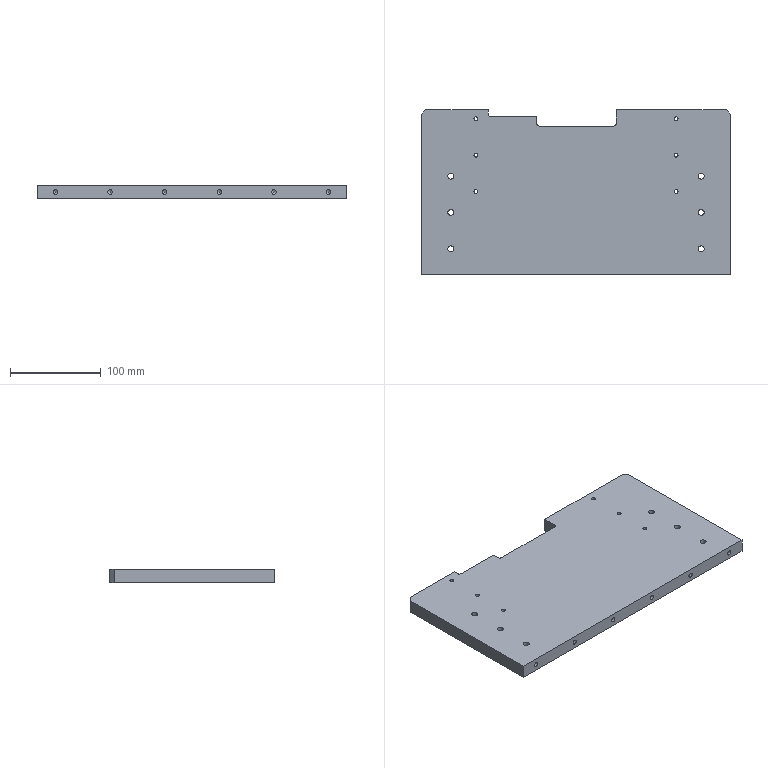Part | NX | 1 solid | 63 faces | box 340 x 181 x 15 mm | volume 882537 mm3 | cylinder 32 | plane 20 | cone 11 | commonest cylinder face diameters 5 x11 4.2 x6 6.6 x6 11 x6 6 x3